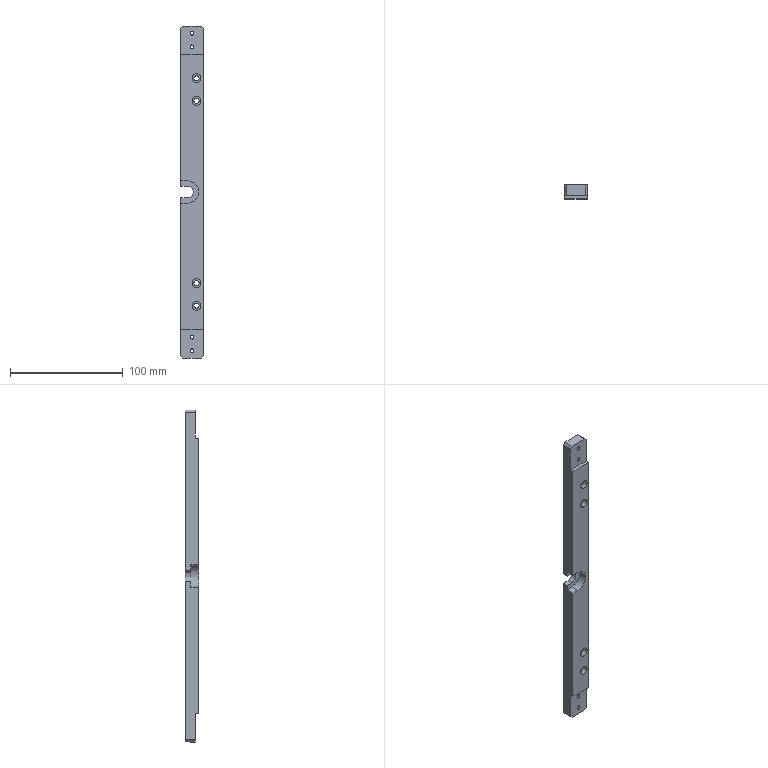Part | SolidWorks | features HoleWzd 3, ICE 3, Cut 2, Chamfer 1, Extrusion 1 | 1 solid | 64 faces | box 20 x 12 x 295 mm | volume 61579 mm3 | cylinder 32 | plane 32 | commonest cylinder face diameters 3.3 x8 4.5 x8 8 x8 3 x6 10.1 x1 20 x1